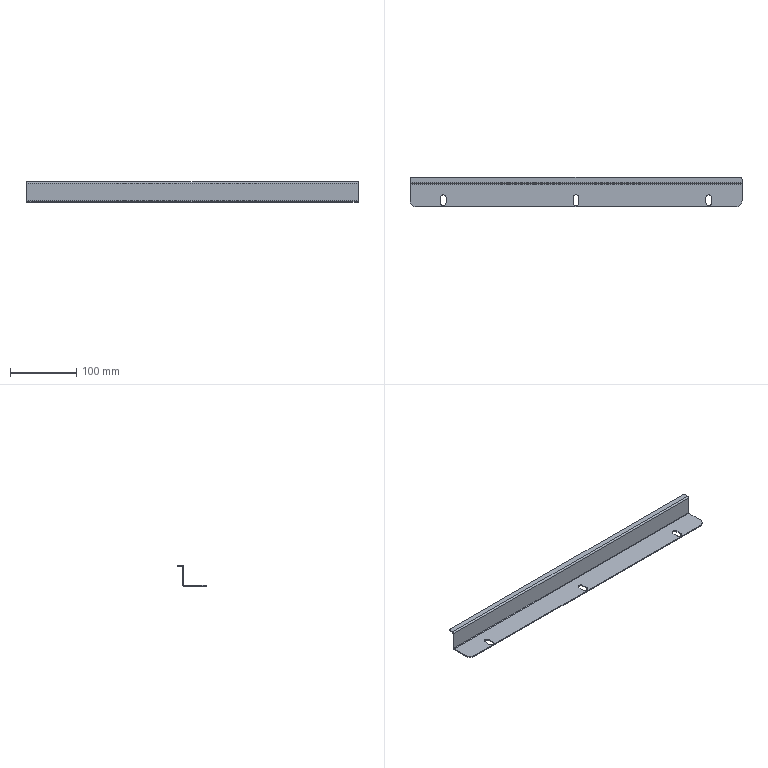Part | SolidWorks | features BaseBody 1 | 1 solid | 38 faces | box 500 x 45 x 31.5 mm | volume 54661 mm3 | plane 24 | cylinder 14 | commonest cylinder face diameters 8.5 x6 1.473 x2 4.473 x2 6 x2 20 x2
STEP:
#1=CARTESIAN_POINT('',(250.,19.,27.763));
#2=VERTEX_POINT('',#1);
#3=CARTESIAN_POINT('',(250.,17.5,27.763));
#4=VERTEX_POINT('',#3);
#5=CARTESIAN_POINT('',(250.,19.,27.763));
#6=DIRECTION('',(0.,-1.,0.));
#7=VECTOR('',#6,1000.);
#8=LINE('',#5,#7);
#9=EDGE_CURVE('',#2,#4,#8,.T.);
#10=ORIENTED_EDGE('',*,*,#9,.T.);
#11=CARTESIAN_POINT('',(250.,17.5,0.7366));
#12=VERTEX_POINT('',#11);
#13=CARTESIAN_POINT('',(250.,17.5,0.));
#14=DIRECTION('',(0.,0.,-1.));
#15=VECTOR('',#14,1000.);
#16=LINE('',#13,#15);
#17=EDGE_CURVE('',#4,#12,#16,.T.);
#18=ORIENTED_EDGE('',*,*,#17,.T.);
#19=CARTESIAN_POINT('',(250.,19.,0.7366));
#20=VERTEX_POINT('',#19);
#21=CARTESIAN_POINT('',(250.,17.5,0.7366));
#22=DIRECTION('',(0.,1.,0.));
#23=VECTOR('',#22,1000.);
#24=LINE('',#21,#23);
#25=EDGE_CURVE('',#12,#20,#24,.T.);
#26=ORIENTED_EDGE('',*,*,#25,.T.);
#27=CARTESIAN_POINT('',(250.,19.,0.));
#28=DIRECTION('',(0.,0.,-1.));
#29=VECTOR('',#28,1000.);
#30=LINE('',#27,#29);
#31=EDGE_CURVE('',#2,#20,#30,.T.);
#32=ORIENTED_EDGE('',*,*,#31,.F.);
#33=EDGE_LOOP('',(#10,#18,#26,#32));
#34=FACE_OUTER_BOUND('',#33,.T.);
#35=CARTESIAN_POINT('',(250.,19.,0.));
#36=DIRECTION('',(-1.,0.,0.));
#37=DIRECTION('',(0.,0.,1.));
#38=AXIS2_PLACEMENT_3D('',#35,#36,#37);
#39=PLANE('',#38);
#40=ADVANCED_FACE('',(#34),#39,.F.);
#41=CARTESIAN_POINT('',(-250.,19.,27.763));
#42=VERTEX_POINT('',#41);
#43=CARTESIAN_POINT('',(-250.,17.5,27.763));
#44=VERTEX_POINT('',#43);
#45=CARTESIAN_POINT('',(-250.,19.,27.763));
#46=DIRECTION('',(0.,-1.,0.));
#47=VECTOR('',#46,1000.);
#48=LINE('',#45,#47);
#49=EDGE_CURVE('',#42,#44,#48,.T.);
#50=ORIENTED_EDGE('',*,*,#49,.F.);
#51=CARTESIAN_POINT('',(-250.,19.,0.7366));
#52=VERTEX_POINT('',#51);
#53=CARTESIAN_POINT('',(-250.,19.,28.5));
#54=DIRECTION('',(0.,0.,1.));
#55=VECTOR('',#54,1000.);
#56=LINE('',#53,#55);
#57=EDGE_CURVE('',#52,#42,#56,.T.);
#58=ORIENTED_EDGE('',*,*,#57,.F.);
#59=CARTESIAN_POINT('',(-250.,17.5,0.7366));
#60=VERTEX_POINT('',#59);
#61=CARTESIAN_POINT('',(-250.,17.5,0.7366));
#62=DIRECTION('',(0.,1.,0.));
#63=VECTOR('',#62,1000.);
#64=LINE('',#61,#63);
#65=EDGE_CURVE('',#60,#52,#64,.T.);
#66=ORIENTED_EDGE('',*,*,#65,.F.);
#67=CARTESIAN_POINT('',(-250.,17.5,28.5));
#68=DIRECTION('',(0.,0.,1.));
#69=VECTOR('',#68,1000.);
#70=LINE('',#67,#69);
#71=EDGE_CURVE('',#60,#44,#70,.T.);
#72=ORIENTED_EDGE('',*,*,#71,.T.);
#73=EDGE_LOOP('',(#50,#58,#66,#72));
#74=FACE_OUTER_BOUND('',#73,.T.);
#75=CARTESIAN_POINT('',(-250.,19.,28.5));
#76=DIRECTION('',(1.,0.,0.));
#77=DIRECTION('',(0.,0.,-1.));
#78=AXIS2_PLACEMENT_3D('',#75,#76,#77);
#79=PLANE('',#78);
#80=ADVANCED_FACE('',(#74),#79,.F.);
#81=CARTESIAN_POINT('',(250.,19.,27.763));
#82=DIRECTION('',(-1.,0.,0.));
#83=VECTOR('',#82,1000.);
#84=LINE('',#81,#83);
#85=EDGE_CURVE('',#2,#42,#84,.T.);
#86=ORIENTED_EDGE('',*,*,#85,.F.);
#87=ORIENTED_EDGE('',*,*,#31,.T.);
#88=CARTESIAN_POINT('',(250.,19.,0.7366));
#89=DIRECTION('',(1.,0.,0.));
#90=VECTOR('',#89,1000.);
#91=LINE('',#88,#90);
#92=EDGE_CURVE('',#52,#20,#91,.T.);
#93=ORIENTED_EDGE('',*,*,#92,.F.);
#94=ORIENTED_EDGE('',*,*,#57,.T.);
#95=EDGE_LOOP('',(#86,#87,#93,#94));
#96=FACE_OUTER_BOUND('',#95,.T.);
#97=CARTESIAN_POINT('',(250.,19.,28.5));
#98=DIRECTION('',(0.,-1.,0.));
#99=DIRECTION('',(0.,0.,-1.));
#100=AXIS2_PLACEMENT_3D('',#97,#98,#99);
#101=PLANE('',#100);
#102=ADVANCED_FACE('',(#96),#101,.F.);
#103=ORIENTED_EDGE('',*,*,#17,.F.);
#104=CARTESIAN_POINT('',(250.,17.5,27.763));
#105=DIRECTION('',(-1.,0.,0.));
#106=VECTOR('',#105,1000.);
#107=LINE('',#104,#106);
#108=EDGE_CURVE('',#4,#44,#107,.T.);
#109=ORIENTED_EDGE('',*,*,#108,.T.);
#110=ORIENTED_EDGE('',*,*,#71,.F.);
#111=CARTESIAN_POINT('',(250.,17.5,0.7366));
#112=DIRECTION('',(-1.,0.,0.));
#113=VECTOR('',#112,1000.);
#114=LINE('',#111,#113);
#115=EDGE_CURVE('',#12,#60,#114,.T.);
#116=ORIENTED_EDGE('',*,*,#115,.F.);
#117=EDGE_LOOP('',(#103,#109,#110,#116));
#118=FACE_OUTER_BOUND('',#117,.T.);
#119=CARTESIAN_POINT('',(250.,17.5,28.5));
#120=DIRECTION('',(0.,-1.,0.));
#121=DIRECTION('',(0.,0.,-1.));
#122=AXIS2_PLACEMENT_3D('',#119,#120,#121);
#123=PLANE('',#122);
#124=ADVANCED_FACE('',(#118),#123,.T.);
#125=CARTESIAN_POINT('',(-250.,16.763,-1.5));
#126=VERTEX_POINT('',#125);
#127=CARTESIAN_POINT('',(-250.,-7.5,-1.5));
#128=VERTEX_POINT('',#127);
#129=CARTESIAN_POINT('',(-250.,17.5,-1.5));
#130=DIRECTION('',(0.,-1.,0.));
#131=VECTOR('',#130,1000.);
#132=LINE('',#129,#131);
#133=EDGE_CURVE('',#126,#128,#132,.T.);
#134=ORIENTED_EDGE('',*,*,#133,.T.);
#135=CARTESIAN_POINT('',(-250.,-7.5,0.));
#136=VERTEX_POINT('',#135);
#137=CARTESIAN_POINT('',(-250.,-7.5,-1.5));
#138=DIRECTION('',(0.,0.,1.));
#139=VECTOR('',#138,1000.);
#140=LINE('',#137,#139);
#141=EDGE_CURVE('',#128,#136,#140,.T.);
#142=ORIENTED_EDGE('',*,*,#141,.T.);
#143=CARTESIAN_POINT('',(-250.,16.763,0.));
#144=VERTEX_POINT('',#143);
#145=CARTESIAN_POINT('',(-250.,17.5,0.));
#146=DIRECTION('',(0.,-1.,0.));
#147=VECTOR('',#146,1000.);
#148=LINE('',#145,#147);
#149=EDGE_CURVE('',#144,#136,#148,.T.);
#150=ORIENTED_EDGE('',*,*,#149,.F.);
#151=CARTESIAN_POINT('',(-250.,16.763,0.));
#152=DIRECTION('',(0.,0.,-1.));
#153=VECTOR('',#152,1000.);
#154=LINE('',#151,#153);
#155=EDGE_CURVE('',#144,#126,#154,.T.);
#156=ORIENTED_EDGE('',*,*,#155,.T.);
#157=EDGE_LOOP('',(#134,#142,#150,#156));
#158=FACE_OUTER_BOUND('',#157,.T.);
#159=CARTESIAN_POINT('',(-250.,17.5,-1.5));
#160=DIRECTION('',(-1.,0.,0.));
#161=DIRECTION('',(0.,0.,1.));
#162=AXIS2_PLACEMENT_3D('',#159,#160,#161);
#163=PLANE('',#162);
#164=ADVANCED_FACE('',(#158),#163,.T.);
#165=CARTESIAN_POINT('',(4.25,-11.5,-1.5));
#166=VERTEX_POINT('',#165);
#167=CARTESIAN_POINT('',(-4.25,-11.5,-1.5));
#168=VERTEX_POINT('',#167);
#169=CARTESIAN_POINT('',(0.,-11.5,-1.5));
#170=DIRECTION('',(0.,0.,-1.));
#171=DIRECTION('',(-1.,0.,0.));
#172=AXIS2_PLACEMENT_3D('',#169,#170,#171);
#173=CIRCLE('',#172,4.25);
#174=EDGE_CURVE('',#166,#168,#173,.T.);
#175=ORIENTED_EDGE('',*,*,#174,.F.);
#176=CARTESIAN_POINT('',(4.25,-3.5,-1.5));
#177=VERTEX_POINT('',#176);
#178=CARTESIAN_POINT('',(4.25,-17.5,-1.5));
#179=DIRECTION('',(0.,-1.,0.));
#180=VECTOR('',#179,1000.);
#181=LINE('',#178,#180);
#182=EDGE_CURVE('',#177,#166,#181,.T.);
#183=ORIENTED_EDGE('',*,*,#182,.F.);
#184=CARTESIAN_POINT('',(-4.25,-3.5,-1.5));
#185=VERTEX_POINT('',#184);
#186=CARTESIAN_POINT('',(0.,-3.5,-1.5));
#187=DIRECTION('',(0.,0.,-1.));
#188=DIRECTION('',(-1.,0.,0.));
#189=AXIS2_PLACEMENT_3D('',#186,#187,#188);
#190=CIRCLE('',#189,4.25);
#191=EDGE_CURVE('',#185,#177,#190,.T.);
#192=ORIENTED_EDGE('',*,*,#191,.F.);
#193=CARTESIAN_POINT('',(-4.25,-17.5,-1.5));
#194=DIRECTION('',(0.,1.,0.));
#195=VECTOR('',#194,1000.);
#196=LINE('',#193,#195);
#197=EDGE_CURVE('',#168,#185,#196,.T.);
#198=ORIENTED_EDGE('',*,*,#197,.F.);
#199=EDGE_LOOP('',(#175,#183,#192,#198));
#200=FACE_BOUND('',#199,.T.);
#201=CARTESIAN_POINT('',(195.75,-3.5,-1.5));
#202=VERTEX_POINT('',#201);
#203=CARTESIAN_POINT('',(204.25,-3.5,-1.5));
#204=VERTEX_POINT('',#203);
#205=CARTESIAN_POINT('',(200.,-3.5,-1.5));
#206=DIRECTION('',(0.,0.,-1.));
#207=DIRECTION('',(-1.,0.,0.));
#208=AXIS2_PLACEMENT_3D('',#205,#206,#207);
#209=CIRCLE('',#208,4.25);
#210=EDGE_CURVE('',#202,#204,#209,.T.);
#211=ORIENTED_EDGE('',*,*,#210,.F.);
#212=CARTESIAN_POINT('',(195.75,-11.5,-1.5));
#213=VERTEX_POINT('',#212);
#214=CARTESIAN_POINT('',(195.75,-17.5,-1.5));
#215=DIRECTION('',(0.,1.,0.));
#216=VECTOR('',#215,1000.);
#217=LINE('',#214,#216);
#218=EDGE_CURVE('',#213,#202,#217,.T.);
#219=ORIENTED_EDGE('',*,*,#218,.F.);
#220=CARTESIAN_POINT('',(204.25,-11.5,-1.5));
#221=VERTEX_POINT('',#220);
#222=CARTESIAN_POINT('',(200.,-11.5,-1.5));
#223=DIRECTION('',(0.,0.,-1.));
#224=DIRECTION('',(-1.,0.,0.));
#225=AXIS2_PLACEMENT_3D('',#222,#223,#224);
#226=CIRCLE('',#225,4.25);
#227=EDGE_CURVE('',#221,#213,#226,.T.);
#228=ORIENTED_EDGE('',*,*,#227,.F.);
#229=CARTESIAN_POINT('',(204.25,-17.5,-1.5));
#230=DIRECTION('',(0.,-1.,0.));
#231=VECTOR('',#230,1000.);
#232=LINE('',#229,#231);
#233=EDGE_CURVE('',#204,#221,#232,.T.);
#234=ORIENTED_EDGE('',*,*,#233,.F.);
#235=EDGE_LOOP('',(#211,#219,#228,#234));
#236=FACE_BOUND('',#235,.T.);
#237=CARTESIAN_POINT('',(-204.25,-3.5,-1.5));
#238=VERTEX_POINT('',#237);
#239=CARTESIAN_POINT('',(-195.75,-3.5,-1.5));
#240=VERTEX_POINT('',#239);
#241=CARTESIAN_POINT('',(-200.,-3.5,-1.5));
#242=DIRECTION('',(0.,0.,-1.));
#243=DIRECTION('',(-1.,0.,0.));
#244=AXIS2_PLACEMENT_3D('',#241,#242,#243);
#245=CIRCLE('',#244,4.25);
#246=EDGE_CURVE('',#238,#240,#245,.T.);
#247=ORIENTED_EDGE('',*,*,#246,.F.);
#248=CARTESIAN_POINT('',(-204.25,-11.5,-1.5));
#249=VERTEX_POINT('',#248);
#250=CARTESIAN_POINT('',(-204.25,-17.5,-1.5));
#251=DIRECTION('',(0.,1.,0.));
#252=VECTOR('',#251,1000.);
#253=LINE('',#250,#252);
#254=EDGE_CURVE('',#249,#238,#253,.T.);
#255=ORIENTED_EDGE('',*,*,#254,.F.);
#256=CARTESIAN_POINT('',(-195.75,-11.5,-1.5));
#257=VERTEX_POINT('',#256);
#258=CARTESIAN_POINT('',(-200.,-11.5,-1.5));
#259=DIRECTION('',(0.,0.,-1.));
#260=DIRECTION('',(-1.,0.,0.));
#261=AXIS2_PLACEMENT_3D('',#258,#259,#260);
#262=CIRCLE('',#261,4.25);
#263=EDGE_CURVE('',#257,#249,#262,.T.);
#264=ORIENTED_EDGE('',*,*,#263,.F.);
#265=CARTESIAN_POINT('',(-195.75,-17.5,-1.5));
#266=DIRECTION('',(0.,-1.,0.));
#267=VECTOR('',#266,1000.);
#268=LINE('',#265,#267);
#269=EDGE_CURVE('',#240,#257,#268,.T.);
#270=ORIENTED_EDGE('',*,*,#269,.F.);
#271=EDGE_LOOP('',(#247,#255,#264,#270));
#272=FACE_BOUND('',#271,.T.);
#273=CARTESIAN_POINT('',(250.,-7.5,-1.5));
#274=VERTEX_POINT('',#273);
#275=CARTESIAN_POINT('',(250.,16.763,-1.5));
#276=VERTEX_POINT('',#275);
#277=CARTESIAN_POINT('',(250.,17.5,-1.5));
#278=DIRECTION('',(0.,1.,0.));
#279=VECTOR('',#278,1000.);
#280=LINE('',#277,#279);
#281=EDGE_CURVE('',#274,#276,#280,.T.);
#282=ORIENTED_EDGE('',*,*,#281,.F.);
#283=CARTESIAN_POINT('',(240.,-17.5,-1.5));
#284=VERTEX_POINT('',#283);
#285=CARTESIAN_POINT('',(240.,-7.5,-1.5));
#286=DIRECTION('',(0.,0.,-1.));
#287=DIRECTION('',(-1.,0.,0.));
#288=AXIS2_PLACEMENT_3D('',#285,#286,#287);
#289=CIRCLE('',#288,10.);
#290=EDGE_CURVE('',#274,#284,#289,.T.);
#291=ORIENTED_EDGE('',*,*,#290,.T.);
#292=CARTESIAN_POINT('',(-240.,-17.5,-1.5));
#293=VERTEX_POINT('',#292);
#294=CARTESIAN_POINT('',(250.,-17.5,-1.5));
#295=DIRECTION('',(1.,0.,0.));
#296=VECTOR('',#295,1000.);
#297=LINE('',#294,#296);
#298=EDGE_CURVE('',#293,#284,#297,.T.);
#299=ORIENTED_EDGE('',*,*,#298,.F.);
#300=CARTESIAN_POINT('',(-240.,-7.5,-1.5));
#301=DIRECTION('',(0.,0.,-1.));
#302=DIRECTION('',(-1.,0.,0.));
#303=AXIS2_PLACEMENT_3D('',#300,#301,#302);
#304=CIRCLE('',#303,10.);
#305=EDGE_CURVE('',#293,#128,#304,.T.);
#306=ORIENTED_EDGE('',*,*,#305,.T.);
#307=ORIENTED_EDGE('',*,*,#133,.F.);
#308=CARTESIAN_POINT('',(-250.,16.763,-1.5));
#309=DIRECTION('',(1.,0.,0.));
#310=VECTOR('',#309,1000.);
#311=LINE('',#308,#310);
#312=EDGE_CURVE('',#126,#276,#311,.T.);
#313=ORIENTED_EDGE('',*,*,#312,.T.);
#314=EDGE_LOOP('',(#282,#291,#299,#306,#307,#313));
#315=FACE_OUTER_BOUND('',#314,.T.);
#316=CARTESIAN_POINT('',(-250.,-17.5,-1.5));
#317=DIRECTION('',(0.,0.,-1.));
#318=DIRECTION('',(-1.,0.,0.));
#319=AXIS2_PLACEMENT_3D('',#316,#317,#318);
#320=PLANE('',#319);
#321=ADVANCED_FACE('',(#200,#236,#272,#315),#320,.T.);
#322=CARTESIAN_POINT('',(4.25,-11.5,0.));
#323=VERTEX_POINT('',#322);
#324=CARTESIAN_POINT('',(4.25,-3.5,0.));
#325=VERTEX_POINT('',#324);
#326=CARTESIAN_POINT('',(4.25,-11.5,0.));
#327=DIRECTION('',(0.,1.,0.));
#328=VECTOR('',#327,1000.);
#329=LINE('',#326,#328);
#330=EDGE_CURVE('',#323,#325,#329,.T.);
#331=ORIENTED_EDGE('',*,*,#330,.F.);
#332=CARTESIAN_POINT('',(-4.25,-11.5,0.));
#333=VERTEX_POINT('',#332);
#334=CARTESIAN_POINT('',(0.,-11.5,0.));
#335=DIRECTION('',(0.,0.,1.));
#336=DIRECTION('',(1.,0.,0.));
#337=AXIS2_PLACEMENT_3D('',#334,#335,#336);
#338=CIRCLE('',#337,4.25);
#339=EDGE_CURVE('',#333,#323,#338,.T.);
#340=ORIENTED_EDGE('',*,*,#339,.F.);
#341=CARTESIAN_POINT('',(-4.25,-3.5,0.));
#342=VERTEX_POINT('',#341);
#343=CARTESIAN_POINT('',(-4.25,-11.5,0.));
#344=DIRECTION('',(0.,-1.,0.));
#345=VECTOR('',#344,1000.);
#346=LINE('',#343,#345);
#347=EDGE_CURVE('',#342,#333,#346,.T.);
#348=ORIENTED_EDGE('',*,*,#347,.F.);
#349=CARTESIAN_POINT('',(0.,-3.5,0.));
#350=DIRECTION('',(0.,0.,1.));
#351=DIRECTION('',(1.,0.,0.));
#352=AXIS2_PLACEMENT_3D('',#349,#350,#351);
#353=CIRCLE('',#352,4.25);
#354=EDGE_CURVE('',#325,#342,#353,.T.);
#355=ORIENTED_EDGE('',*,*,#354,.F.);
#356=EDGE_LOOP('',(#331,#340,#348,#355));
#357=FACE_BOUND('',#356,.T.);
#358=CARTESIAN_POINT('',(195.75,-3.5,0.));
#359=VERTEX_POINT('',#358);
#360=CARTESIAN_POINT('',(195.75,-11.5,0.));
#361=VERTEX_POINT('',#360);
#362=CARTESIAN_POINT('',(195.75,-3.5,0.));
#363=DIRECTION('',(0.,-1.,0.));
#364=VECTOR('',#363,1000.);
#365=LINE('',#362,#364);
#366=EDGE_CURVE('',#359,#361,#365,.T.);
#367=ORIENTED_EDGE('',*,*,#366,.F.);
#368=CARTESIAN_POINT('',(204.25,-3.5,0.));
#369=VERTEX_POINT('',#368);
#370=CARTESIAN_POINT('',(200.,-3.5,0.));
#371=DIRECTION('',(0.,0.,1.));
#372=DIRECTION('',(-1.,0.,0.));
#373=AXIS2_PLACEMENT_3D('',#370,#371,#372);
#374=CIRCLE('',#373,4.25);
#375=EDGE_CURVE('',#369,#359,#374,.T.);
#376=ORIENTED_EDGE('',*,*,#375,.F.);
#377=CARTESIAN_POINT('',(204.25,-11.5,0.));
#378=VERTEX_POINT('',#377);
#379=CARTESIAN_POINT('',(204.25,-3.5,0.));
#380=DIRECTION('',(0.,1.,0.));
#381=VECTOR('',#380,1000.);
#382=LINE('',#379,#381);
#383=EDGE_CURVE('',#378,#369,#382,.T.);
#384=ORIENTED_EDGE('',*,*,#383,.F.);
#385=CARTESIAN_POINT('',(200.,-11.5,0.));
#386=DIRECTION('',(0.,0.,1.));
#387=DIRECTION('',(-1.,0.,0.));
#388=AXIS2_PLACEMENT_3D('',#385,#386,#387);
#389=CIRCLE('',#388,4.25);
#390=EDGE_CURVE('',#361,#378,#389,.T.);
#391=ORIENTED_EDGE('',*,*,#390,.F.);
#392=EDGE_LOOP('',(#367,#376,#384,#391));
#393=FACE_BOUND('',#392,.T.);
#394=CARTESIAN_POINT('',(-204.25,-3.5,0.));
#395=VERTEX_POINT('',#394);
#396=CARTESIAN_POINT('',(-204.25,-11.5,0.));
#397=VERTEX_POINT('',#396);
#398=CARTESIAN_POINT('',(-204.25,-3.5,0.));
#399=DIRECTION('',(0.,-1.,0.));
#400=VECTOR('',#399,1000.);
#401=LINE('',#398,#400);
#402=EDGE_CURVE('',#395,#397,#401,.T.);
#403=ORIENTED_EDGE('',*,*,#402,.F.);
#404=CARTESIAN_POINT('',(-195.75,-3.5,0.));
#405=VERTEX_POINT('',#404);
#406=CARTESIAN_POINT('',(-200.,-3.5,0.));
#407=DIRECTION('',(0.,0.,1.));
#408=DIRECTION('',(1.,0.,0.));
#409=AXIS2_PLACEMENT_3D('',#406,#407,#408);
#410=CIRCLE('',#409,4.25);
#411=EDGE_CURVE('',#405,#395,#410,.T.);
#412=ORIENTED_EDGE('',*,*,#411,.F.);
#413=CARTESIAN_POINT('',(-195.75,-11.5,0.));
#414=VERTEX_POINT('',#413);
#415=CARTESIAN_POINT('',(-195.75,-3.5,0.));
#416=DIRECTION('',(0.,1.,0.));
#417=VECTOR('',#416,1000.);
#418=LINE('',#415,#417);
#419=EDGE_CURVE('',#414,#405,#418,.T.);
#420=ORIENTED_EDGE('',*,*,#419,.F.);
#421=CARTESIAN_POINT('',(-200.,-11.5,0.));
#422=DIRECTION('',(0.,0.,1.));
#423=DIRECTION('',(1.,0.,0.));
#424=AXIS2_PLACEMENT_3D('',#421,#422,#423);
#425=CIRCLE('',#424,4.25);
#426=EDGE_CURVE('',#397,#414,#425,.T.);
#427=ORIENTED_EDGE('',*,*,#426,.F.);
#428=EDGE_LOOP('',(#403,#412,#420,#427));
#429=FACE_BOUND('',#428,.T.);
#430=CARTESIAN_POINT('',(-240.,-17.5,0.));
#431=VERTEX_POINT('',#430);
#432=CARTESIAN_POINT('',(240.,-17.5,0.));
#433=VERTEX_POINT('',#432);
#434=CARTESIAN_POINT('',(250.,-17.5,0.));
#435=DIRECTION('',(1.,0.,0.));
#436=VECTOR('',#435,1000.);
#437=LINE('',#434,#436);
#438=EDGE_CURVE('',#431,#433,#437,.T.);
#439=ORIENTED_EDGE('',*,*,#438,.T.);
#440=CARTESIAN_POINT('',(250.,-7.5,0.));
#441=VERTEX_POINT('',#440);
#442=CARTESIAN_POINT('',(240.,-7.5,0.));
#443=DIRECTION('',(0.,0.,1.));
#444=DIRECTION('',(-1.,0.,0.));
#445=AXIS2_PLACEMENT_3D('',#442,#443,#444);
#446=CIRCLE('',#445,10.);
#447=EDGE_CURVE('',#433,#441,#446,.T.);
#448=ORIENTED_EDGE('',*,*,#447,.T.);
#449=CARTESIAN_POINT('',(250.,16.763,0.));
#450=VERTEX_POINT('',#449);
#451=CARTESIAN_POINT('',(250.,17.5,0.));
#452=DIRECTION('',(0.,1.,0.));
#453=VECTOR('',#452,1000.);
#454=LINE('',#451,#453);
#455=EDGE_CURVE('',#441,#450,#454,.T.);
#456=ORIENTED_EDGE('',*,*,#455,.T.);
#457=CARTESIAN_POINT('',(-250.,16.763,0.));
#458=DIRECTION('',(1.,0.,0.));
#459=VECTOR('',#458,1000.);
#460=LINE('',#457,#459);
#461=EDGE_CURVE('',#144,#450,#460,.T.);
#462=ORIENTED_EDGE('',*,*,#461,.F.);
#463=ORIENTED_EDGE('',*,*,#149,.T.);
#464=CARTESIAN_POINT('',(-240.,-7.5,0.));
#465=DIRECTION('',(0.,0.,1.));
#466=DIRECTION('',(-1.,0.,0.));
#467=AXIS2_PLACEMENT_3D('',#464,#465,#466);
#468=CIRCLE('',#467,10.);
#469=EDGE_CURVE('',#136,#431,#468,.T.);
#470=ORIENTED_EDGE('',*,*,#469,.T.);
#471=EDGE_LOOP('',(#439,#448,#456,#462,#463,#470));
#472=FACE_OUTER_BOUND('',#471,.T.);
#473=CARTESIAN_POINT('',(-250.,-17.5,0.));
#474=DIRECTION('',(0.,0.,-1.));
#475=DIRECTION('',(-1.,0.,0.));
#476=AXIS2_PLACEMENT_3D('',#473,#474,#475);
#477=PLANE('',#476);
#478=ADVANCED_FACE('',(#357,#393,#429,#472),#477,.F.);
#479=ORIENTED_EDGE('',*,*,#455,.F.);
#480=CARTESIAN_POINT('',(250.,-7.5,-1.5));
#481=DIRECTION('',(0.,0.,-1.));
#482=VECTOR('',#481,1000.);
#483=LINE('',#480,#482);
#484=EDGE_CURVE('',#441,#274,#483,.T.);
#485=ORIENTED_EDGE('',*,*,#484,.T.);
#486=ORIENTED_EDGE('',*,*,#281,.T.);
#487=CARTESIAN_POINT('',(250.,16.763,0.));
#488=DIRECTION('',(0.,0.,-1.));
#489=VECTOR('',#488,1000.);
#490=LINE('',#487,#489);
#491=EDGE_CURVE('',#450,#276,#490,.T.);
#492=ORIENTED_EDGE('',*,*,#491,.F.);
#493=EDGE_LOOP('',(#479,#485,#486,#492));
#494=FACE_OUTER_BOUND('',#493,.T.);
#495=CARTESIAN_POINT('',(250.,17.5,-1.5));
#496=DIRECTION('',(1.,0.,0.));
#497=DIRECTION('',(0.,1.,0.));
#498=AXIS2_PLACEMENT_3D('',#495,#496,#497);
#499=PLANE('',#498);
#500=ADVANCED_FACE('',(#494),#499,.T.);
#501=ORIENTED_EDGE('',*,*,#298,.T.);
#502=CARTESIAN_POINT('',(240.,-17.5,-1.5));
#503=DIRECTION('',(0.,0.,1.));
#504=VECTOR('',#503,1000.);
#505=LINE('',#502,#504);
#506=EDGE_CURVE('',#284,#433,#505,.T.);
#507=ORIENTED_EDGE('',*,*,#506,.T.);
#508=ORIENTED_EDGE('',*,*,#438,.F.);
#509=CARTESIAN_POINT('',(-240.,-17.5,-1.5));
#510=DIRECTION('',(0.,0.,-1.));
#511=VECTOR('',#510,1000.);
#512=LINE('',#509,#511);
#513=EDGE_CURVE('',#431,#293,#512,.T.);
#514=ORIENTED_EDGE('',*,*,#513,.T.);
#515=EDGE_LOOP('',(#501,#507,#508,#514));
#516=FACE_OUTER_BOUND('',#515,.T.);
#517=CARTESIAN_POINT('',(250.,-17.5,-1.5));
#518=DIRECTION('',(0.,-1.,0.));
#519=DIRECTION('',(1.,0.,0.));
#520=AXIS2_PLACEMENT_3D('',#517,#518,#519);
#521=PLANE('',#520);
#522=ADVANCED_FACE('',(#516),#521,.T.);
#523=ORIENTED_EDGE('',*,*,#25,.F.);
#524=CARTESIAN_POINT('',(250.,16.763,0.7366));
#525=DIRECTION('',(1.,0.,0.));
#526=DIRECTION('',(0.,0.,1.));
#527=AXIS2_PLACEMENT_3D('',#524,#525,#526);
#528=CIRCLE('',#527,0.7366);
#529=EDGE_CURVE('',#450,#12,#528,.T.);
#530=ORIENTED_EDGE('',*,*,#529,.F.);
#531=ORIENTED_EDGE('',*,*,#491,.T.);
#532=CARTESIAN_POINT('',(250.,16.763,0.7366));
#533=DIRECTION('',(1.,0.,0.));
#534=DIRECTION('',(0.,0.,1.));
#535=AXIS2_PLACEMENT_3D('',#532,#533,#534);
#536=CIRCLE('',#535,2.237);
#537=EDGE_CURVE('',#276,#20,#536,.T.);
#538=ORIENTED_EDGE('',*,*,#537,.T.);
#539=EDGE_LOOP('',(#523,#530,#531,#538));
#540=FACE_OUTER_BOUND('',#539,.T.);
#541=CARTESIAN_POINT('',(250.,16.763,0.7366));
#542=DIRECTION('',(1.,0.,0.));
#543=DIRECTION('',(0.,0.,-1.));
#544=AXIS2_PLACEMENT_3D('',#541,#542,#543);
#545=PLANE('',#544);
#546=ADVANCED_FACE('',(#540),#545,.T.);
#547=CARTESIAN_POINT('',(-250.,16.763,0.7366));
#548=DIRECTION('',(-1.,0.,0.));
#549=DIRECTION('',(0.,0.,1.));
#550=AXIS2_PLACEMENT_3D('',#547,#548,#549);
#551=CIRCLE('',#550,0.7366);
#552=EDGE_CURVE('',#60,#144,#551,.T.);
#553=ORIENTED_EDGE('',*,*,#552,.F.);
#554=ORIENTED_EDGE('',*,*,#65,.T.);
#555=CARTESIAN_POINT('',(-250.,16.763,0.7366));
#556=DIRECTION('',(-1.,0.,0.));
#557=DIRECTION('',(0.,0.,1.));
#558=AXIS2_PLACEMENT_3D('',#555,#556,#557);
#559=CIRCLE('',#558,2.237);
#560=EDGE_CURVE('',#52,#126,#559,.T.);
#561=ORIENTED_EDGE('',*,*,#560,.T.);
#562=ORIENTED_EDGE('',*,*,#155,.F.);
#563=EDGE_LOOP('',(#553,#554,#561,#562));
#564=FACE_OUTER_BOUND('',#563,.T.);
#565=CARTESIAN_POINT('',(-250.,16.763,0.7366));
#566=DIRECTION('',(1.,0.,0.));
#567=DIRECTION('',(0.,0.,-1.));
#568=AXIS2_PLACEMENT_3D('',#565,#566,#567);
#569=PLANE('',#568);
#570=ADVANCED_FACE('',(#564),#569,.F.);
#571=ORIENTED_EDGE('',*,*,#312,.F.);
#572=ORIENTED_EDGE('',*,*,#560,.F.);
#573=ORIENTED_EDGE('',*,*,#92,.T.);
#574=ORIENTED_EDGE('',*,*,#537,.F.);
#575=EDGE_LOOP('',(#571,#572,#573,#574));
#576=FACE_OUTER_BOUND('',#575,.T.);
#577=CARTESIAN_POINT('',(-250.,16.763,0.7366));
#578=DIRECTION('',(-1.,0.,0.));
#579=DIRECTION('',(0.,1.,0.));
#580=AXIS2_PLACEMENT_3D('',#577,#578,#579);
#581=CYLINDRICAL_SURFACE('',#580,2.237);
#582=ADVANCED_FACE('',(#576),#581,.T.);
#583=ORIENTED_EDGE('',*,*,#461,.T.);
#584=ORIENTED_EDGE('',*,*,#529,.T.);
#585=ORIENTED_EDGE('',*,*,#115,.T.);
#586=ORIENTED_EDGE('',*,*,#552,.T.);
#587=EDGE_LOOP('',(#583,#584,#585,#586));
#588=FACE_OUTER_BOUND('',#587,.T.);
#589=CARTESIAN_POINT('',(-250.,16.763,0.7366));
#590=DIRECTION('',(-1.,0.,0.));
#591=DIRECTION('',(0.,1.,0.));
#592=AXIS2_PLACEMENT_3D('',#589,#590,#591);
#593=CYLINDRICAL_SURFACE('',#592,0.7366);
#594=ADVANCED_FACE('',(#588),#593,.F.);
#595=CARTESIAN_POINT('',(-250.,19.737,28.5));
#596=VERTEX_POINT('',#595);
#597=CARTESIAN_POINT('',(-250.,19.737,30.));
#598=VERTEX_POINT('',#597);
#599=CARTESIAN_POINT('',(-250.,19.737,28.5));
#600=DIRECTION('',(0.,0.,1.));
#601=VECTOR('',#600,1000.);
#602=LINE('',#599,#601);
#603=EDGE_CURVE('',#596,#598,#602,.T.);
#604=ORIENTED_EDGE('',*,*,#603,.F.);
#605=CARTESIAN_POINT('',(-250.,19.737,27.763));
#606=DIRECTION('',(-1.,0.,0.));
#607=DIRECTION('',(0.,0.,-1.));
#608=AXIS2_PLACEMENT_3D('',#605,#606,#607);
#609=CIRCLE('',#608,0.7366);
#610=EDGE_CURVE('',#42,#596,#609,.T.);
#611=ORIENTED_EDGE('',*,*,#610,.F.);
#612=ORIENTED_EDGE('',*,*,#49,.T.);
#613=CARTESIAN_POINT('',(-250.,19.737,27.763));
#614=DIRECTION('',(-1.,0.,0.));
#615=DIRECTION('',(0.,0.,-1.));
#616=AXIS2_PLACEMENT_3D('',#613,#614,#615);
#617=CIRCLE('',#616,2.237);
#618=EDGE_CURVE('',#44,#598,#617,.T.);
#619=ORIENTED_EDGE('',*,*,#618,.T.);
#620=EDGE_LOOP('',(#604,#611,#612,#619));
#621=FACE_OUTER_BOUND('',#620,.T.);
#622=CARTESIAN_POINT('',(-250.,19.737,27.763));
#623=DIRECTION('',(-1.,0.,0.));
#624=DIRECTION('',(0.,0.,1.));
#625=AXIS2_PLACEMENT_3D('',#622,#623,#624);
#626=PLANE('',#625);
#627=ADVANCED_FACE('',(#621),#626,.T.);
#628=CARTESIAN_POINT('',(250.,19.737,28.5));
#629=VERTEX_POINT('',#628);
#630=CARTESIAN_POINT('',(250.,19.737,27.763));
#631=DIRECTION('',(1.,0.,0.));
#632=DIRECTION('',(0.,0.,-1.));
#633=AXIS2_PLACEMENT_3D('',#630,#631,#632);
#634=CIRCLE('',#633,0.7366);
#635=EDGE_CURVE('',#629,#2,#634,.T.);
#636=ORIENTED_EDGE('',*,*,#635,.F.);
#637=CARTESIAN_POINT('',(250.,19.737,30.));
#638=VERTEX_POINT('',#637);
#639=CARTESIAN_POINT('',(250.,19.737,28.5));
#640=DIRECTION('',(0.,0.,1.));
#641=VECTOR('',#640,1000.);
#642=LINE('',#639,#641);
#643=EDGE_CURVE('',#629,#638,#642,.T.);
#644=ORIENTED_EDGE('',*,*,#643,.T.);
#645=CARTESIAN_POINT('',(250.,19.737,27.763));
#646=DIRECTION('',(1.,0.,0.));
#647=DIRECTION('',(0.,0.,-1.));
#648=AXIS2_PLACEMENT_3D('',#645,#646,#647);
#649=CIRCLE('',#648,2.237);
#650=EDGE_CURVE('',#638,#4,#649,.T.);
#651=ORIENTED_EDGE('',*,*,#650,.T.);
#652=ORIENTED_EDGE('',*,*,#9,.F.);
#653=EDGE_LOOP('',(#636,#644,#651,#652));
#654=FACE_OUTER_BOUND('',#653,.T.);
#655=CARTESIAN_POINT('',(250.,19.737,27.763));
#656=DIRECTION('',(-1.,0.,0.));
#657=DIRECTION('',(0.,0.,1.));
#658=AXIS2_PLACEMENT_3D('',#655,#656,#657);
#659=PLANE('',#658);
#660=ADVANCED_FACE('',(#654),#659,.F.);
#661=ORIENTED_EDGE('',*,*,#108,.F.);
#662=ORIENTED_EDGE('',*,*,#650,.F.);
#663=CARTESIAN_POINT('',(-250.,19.737,30.));
#664=DIRECTION('',(-1.,0.,0.));
#665=VECTOR('',#664,1000.);
#666=LINE('',#663,#665);
#667=EDGE_CURVE('',#638,#598,#666,.T.);
#668=ORIENTED_EDGE('',*,*,#667,.T.);
#669=ORIENTED_EDGE('',*,*,#618,.F.);
#670=EDGE_LOOP('',(#661,#662,#668,#669));
#671=FACE_OUTER_BOUND('',#670,.T.);
#672=CARTESIAN_POINT('',(250.,19.737,27.763));
#673=DIRECTION('',(1.,0.,0.));
#674=DIRECTION('',(0.,0.,1.));
#675=AXIS2_PLACEMENT_3D('',#672,#673,#674);
#676=CYLINDRICAL_SURFACE('',#675,2.237);
#677=ADVANCED_FACE('',(#671),#676,.T.);
#678=ORIENTED_EDGE('',*,*,#85,.T.);
#679=ORIENTED_EDGE('',*,*,#610,.T.);
#680=CARTESIAN_POINT('',(-250.,19.737,28.5));
#681=DIRECTION('',(1.,0.,0.));
#682=VECTOR('',#681,1000.);
#683=LINE('',#680,#682);
#684=EDGE_CURVE('',#596,#629,#683,.T.);
#685=ORIENTED_EDGE('',*,*,#684,.T.);
#686=ORIENTED_EDGE('',*,*,#635,.T.);
#687=EDGE_LOOP('',(#678,#679,#685,#686));
#688=FACE_OUTER_BOUND('',#687,.T.);
#689=CARTESIAN_POINT('',(250.,19.737,27.763));
#690=DIRECTION('',(1.,0.,0.));
#691=DIRECTION('',(0.,0.,1.));
#692=AXIS2_PLACEMENT_3D('',#689,#690,#691);
#693=CYLINDRICAL_SURFACE('',#692,0.7366);
#694=ADVANCED_FACE('',(#688),#693,.F.);
#695=CARTESIAN_POINT('',(-250.,24.5,30.));
#696=VERTEX_POINT('',#695);
#697=CARTESIAN_POINT('',(-250.,19.,30.));
#698=DIRECTION('',(0.,-1.,0.));
#699=VECTOR('',#698,1000.);
#700=LINE('',#697,#699);
#701=EDGE_CURVE('',#696,#598,#700,.T.);
#702=ORIENTED_EDGE('',*,*,#701,.F.);
#703=CARTESIAN_POINT('',(-250.,24.5,28.5));
#704=VERTEX_POINT('',#703);
#705=CARTESIAN_POINT('',(-250.,24.5,30.));
#706=DIRECTION('',(0.,0.,-1.));
#707=VECTOR('',#706,1000.);
#708=LINE('',#705,#707);
#709=EDGE_CURVE('',#696,#704,#708,.T.);
#710=ORIENTED_EDGE('',*,*,#709,.T.);
#711=CARTESIAN_POINT('',(-250.,19.,28.5));
#712=DIRECTION('',(0.,-1.,0.));
#713=VECTOR('',#712,1000.);
#714=LINE('',#711,#713);
#715=EDGE_CURVE('',#704,#596,#714,.T.);
#716=ORIENTED_EDGE('',*,*,#715,.T.);
#717=ORIENTED_EDGE('',*,*,#603,.T.);
#718=EDGE_LOOP('',(#702,#710,#716,#717));
#719=FACE_OUTER_BOUND('',#718,.T.);
#720=CARTESIAN_POINT('',(-250.,19.,30.));
#721=DIRECTION('',(1.,0.,0.));
#722=DIRECTION('',(0.,0.,-1.));
#723=AXIS2_PLACEMENT_3D('',#720,#721,#722);
#724=PLANE('',#723);
#725=ADVANCED_FACE('',(#719),#724,.F.);
#726=CARTESIAN_POINT('',(250.,24.5,28.5));
#727=VERTEX_POINT('',#726);
#728=CARTESIAN_POINT('',(250.,27.5,28.5));
#729=DIRECTION('',(0.,1.,0.));
#730=VECTOR('',#729,1000.);
#731=LINE('',#728,#730);
#732=EDGE_CURVE('',#629,#727,#731,.T.);
#733=ORIENTED_EDGE('',*,*,#732,.T.);
#734=CARTESIAN_POINT('',(250.,24.5,30.));
#735=VERTEX_POINT('',#734);
#736=CARTESIAN_POINT('',(250.,24.5,30.));
#737=DIRECTION('',(0.,0.,1.));
#738=VECTOR('',#737,1000.);
#739=LINE('',#736,#738);
#740=EDGE_CURVE('',#727,#735,#739,.T.);
#741=ORIENTED_EDGE('',*,*,#740,.T.);
#742=CARTESIAN_POINT('',(250.,27.5,30.));
#743=DIRECTION('',(0.,1.,0.));
#744=VECTOR('',#743,1000.);
#745=LINE('',#742,#744);
#746=EDGE_CURVE('',#638,#735,#745,.T.);
#747=ORIENTED_EDGE('',*,*,#746,.F.);
#748=ORIENTED_EDGE('',*,*,#643,.F.);
#749=EDGE_LOOP('',(#733,#741,#747,#748));
#750=FACE_OUTER_BOUND('',#749,.T.);
#751=CARTESIAN_POINT('',(250.,27.5,30.));
#752=DIRECTION('',(-1.,0.,0.));
#753=DIRECTION('',(0.,0.,1.));
#754=AXIS2_PLACEMENT_3D('',#751,#752,#753);
#755=PLANE('',#754);
#756=ADVANCED_FACE('',(#750),#755,.F.);
#757=ORIENTED_EDGE('',*,*,#746,.T.);
#758=CARTESIAN_POINT('',(247.,27.5,30.));
#759=VERTEX_POINT('',#758);
#760=CARTESIAN_POINT('',(247.,24.5,30.));
#761=DIRECTION('',(0.,0.,1.));
#762=DIRECTION('',(-1.,0.,0.));
#763=AXIS2_PLACEMENT_3D('',#760,#761,#762);
#764=CIRCLE('',#763,3.);
#765=EDGE_CURVE('',#735,#759,#764,.T.);
#766=ORIENTED_EDGE('',*,*,#765,.T.);
#767=CARTESIAN_POINT('',(-247.,27.5,30.));
#768=VERTEX_POINT('',#767);
#769=CARTESIAN_POINT('',(-250.,27.5,30.));
#770=DIRECTION('',(-1.,0.,0.));
#771=VECTOR('',#770,1000.);
#772=LINE('',#769,#771);
#773=EDGE_CURVE('',#759,#768,#772,.T.);
#774=ORIENTED_EDGE('',*,*,#773,.T.);
#775=CARTESIAN_POINT('',(-247.,24.5,30.));
#776=DIRECTION('',(0.,0.,1.));
#777=DIRECTION('',(-1.,0.,0.));
#778=AXIS2_PLACEMENT_3D('',#775,#776,#777);
#779=CIRCLE('',#778,3.);
#780=EDGE_CURVE('',#768,#696,#779,.T.);
#781=ORIENTED_EDGE('',*,*,#780,.T.);
#782=ORIENTED_EDGE('',*,*,#701,.T.);
#783=ORIENTED_EDGE('',*,*,#667,.F.);
#784=EDGE_LOOP('',(#757,#766,#774,#781,#782,#783));
#785=FACE_OUTER_BOUND('',#784,.T.);
#786=CARTESIAN_POINT('',(-250.,27.5,30.));
#787=DIRECTION('',(0.,0.,-1.));
#788=DIRECTION('',(-1.,0.,0.));
#789=AXIS2_PLACEMENT_3D('',#786,#787,#788);
#790=PLANE('',#789);
#791=ADVANCED_FACE('',(#785),#790,.F.);
#792=CARTESIAN_POINT('',(247.,27.5,28.5));
#793=VERTEX_POINT('',#792);
#794=CARTESIAN_POINT('',(-247.,27.5,28.5));
#795=VERTEX_POINT('',#794);
#796=CARTESIAN_POINT('',(-250.,27.5,28.5));
#797=DIRECTION('',(-1.,0.,0.));
#798=VECTOR('',#797,1000.);
#799=LINE('',#796,#798);
#800=EDGE_CURVE('',#793,#795,#799,.T.);
#801=ORIENTED_EDGE('',*,*,#800,.F.);
#802=CARTESIAN_POINT('',(247.,24.5,28.5));
#803=DIRECTION('',(0.,0.,-1.));
#804=DIRECTION('',(-1.,0.,0.));
#805=AXIS2_PLACEMENT_3D('',#802,#803,#804);
#806=CIRCLE('',#805,3.);
#807=EDGE_CURVE('',#793,#727,#806,.T.);
#808=ORIENTED_EDGE('',*,*,#807,.T.);
#809=ORIENTED_EDGE('',*,*,#732,.F.);
#810=ORIENTED_EDGE('',*,*,#684,.F.);
#811=ORIENTED_EDGE('',*,*,#715,.F.);
#812=CARTESIAN_POINT('',(-247.,24.5,28.5));
#813=DIRECTION('',(0.,0.,-1.));
#814=DIRECTION('',(-1.,0.,0.));
#815=AXIS2_PLACEMENT_3D('',#812,#813,#814);
#816=CIRCLE('',#815,3.);
#817=EDGE_CURVE('',#704,#795,#816,.T.);
#818=ORIENTED_EDGE('',*,*,#817,.T.);
#819=EDGE_LOOP('',(#801,#808,#809,#810,#811,#818));
#820=FACE_OUTER_BOUND('',#819,.T.);
#821=CARTESIAN_POINT('',(-250.,27.5,28.5));
#822=DIRECTION('',(0.,0.,-1.));
#823=DIRECTION('',(-1.,0.,0.));
#824=AXIS2_PLACEMENT_3D('',#821,#822,#823);
#825=PLANE('',#824);
#826=ADVANCED_FACE('',(#820),#825,.T.);
#827=ORIENTED_EDGE('',*,*,#773,.F.);
#828=CARTESIAN_POINT('',(247.,27.5,30.));
#829=DIRECTION('',(0.,0.,-1.));
#830=VECTOR('',#829,1000.);
#831=LINE('',#828,#830);
#832=EDGE_CURVE('',#759,#793,#831,.T.);
#833=ORIENTED_EDGE('',*,*,#832,.T.);
#834=ORIENTED_EDGE('',*,*,#800,.T.);
#835=CARTESIAN_POINT('',(-247.,27.5,30.));
#836=DIRECTION('',(0.,0.,1.));
#837=VECTOR('',#836,1000.);
#838=LINE('',#835,#837);
#839=EDGE_CURVE('',#795,#768,#838,.T.);
#840=ORIENTED_EDGE('',*,*,#839,.T.);
#841=EDGE_LOOP('',(#827,#833,#834,#840));
#842=FACE_OUTER_BOUND('',#841,.T.);
#843=CARTESIAN_POINT('',(-250.,27.5,30.));
#844=DIRECTION('',(0.,-1.,0.));
#845=DIRECTION('',(0.,0.,-1.));
#846=AXIS2_PLACEMENT_3D('',#843,#844,#845);
#847=PLANE('',#846);
#848=ADVANCED_FACE('',(#842),#847,.F.);
#849=ORIENTED_EDGE('',*,*,#246,.T.);
#850=CARTESIAN_POINT('',(-195.75,-3.5,-10.));
#851=DIRECTION('',(0.,0.,1.));
#852=VECTOR('',#851,1000.);
#853=LINE('',#850,#852);
#854=EDGE_CURVE('',#240,#405,#853,.T.);
#855=ORIENTED_EDGE('',*,*,#854,.T.);
#856=ORIENTED_EDGE('',*,*,#411,.T.);
#857=CARTESIAN_POINT('',(-204.25,-3.5,-10.));
#858=DIRECTION('',(0.,0.,1.));
#859=VECTOR('',#858,1000.);
#860=LINE('',#857,#859);
#861=EDGE_CURVE('',#238,#395,#860,.T.);
#862=ORIENTED_EDGE('',*,*,#861,.F.);
#863=EDGE_LOOP('',(#849,#855,#856,#862));
#864=FACE_OUTER_BOUND('',#863,.T.);
#865=CARTESIAN_POINT('',(-200.,-3.5,-10.));
#866=DIRECTION('',(0.,0.,1.));
#867=DIRECTION('',(1.,0.,0.));
#868=AXIS2_PLACEMENT_3D('',#865,#866,#867);
#869=CYLINDRICAL_SURFACE('',#868,4.25);
#870=ADVANCED_FACE('',(#864),#869,.F.);
#871=ORIENTED_EDGE('',*,*,#269,.T.);
#872=CARTESIAN_POINT('',(-195.75,-11.5,-10.));
#873=DIRECTION('',(0.,0.,1.));
#874=VECTOR('',#873,1000.);
#875=LINE('',#872,#874);
#876=EDGE_CURVE('',#257,#414,#875,.T.);
#877=ORIENTED_EDGE('',*,*,#876,.T.);
#878=ORIENTED_EDGE('',*,*,#419,.T.);
#879=ORIENTED_EDGE('',*,*,#854,.F.);
#880=EDGE_LOOP('',(#871,#877,#878,#879));
#881=FACE_OUTER_BOUND('',#880,.T.);
#882=CARTESIAN_POINT('',(-195.75,-3.5,-10.));
#883=DIRECTION('',(1.,0.,0.));
#884=DIRECTION('',(0.,0.,-1.));
#885=AXIS2_PLACEMENT_3D('',#882,#883,#884);
#886=PLANE('',#885);
#887=ADVANCED_FACE('',(#881),#886,.F.);
#888=ORIENTED_EDGE('',*,*,#263,.T.);
#889=CARTESIAN_POINT('',(-204.25,-11.5,-10.));
#890=DIRECTION('',(0.,0.,1.));
#891=VECTOR('',#890,1000.);
#892=LINE('',#889,#891);
#893=EDGE_CURVE('',#249,#397,#892,.T.);
#894=ORIENTED_EDGE('',*,*,#893,.T.);
#895=ORIENTED_EDGE('',*,*,#426,.T.);
#896=ORIENTED_EDGE('',*,*,#876,.F.);
#897=EDGE_LOOP('',(#888,#894,#895,#896));
#898=FACE_OUTER_BOUND('',#897,.T.);
#899=CARTESIAN_POINT('',(-200.,-11.5,-10.));
#900=DIRECTION('',(0.,0.,1.));
#901=DIRECTION('',(1.,0.,0.));
#902=AXIS2_PLACEMENT_3D('',#899,#900,#901);
#903=CYLINDRICAL_SURFACE('',#902,4.25);
#904=ADVANCED_FACE('',(#898),#903,.F.);
#905=ORIENTED_EDGE('',*,*,#254,.T.);
#906=ORIENTED_EDGE('',*,*,#861,.T.);
#907=ORIENTED_EDGE('',*,*,#402,.T.);
#908=ORIENTED_EDGE('',*,*,#893,.F.);
#909=EDGE_LOOP('',(#905,#906,#907,#908));
#910=FACE_OUTER_BOUND('',#909,.T.);
#911=CARTESIAN_POINT('',(-204.25,-3.5,-10.));
#912=DIRECTION('',(-1.,0.,0.));
#913=DIRECTION('',(0.,0.,1.));
#914=AXIS2_PLACEMENT_3D('',#911,#912,#913);
#915=PLANE('',#914);
#916=ADVANCED_FACE('',(#910),#915,.F.);
#917=ORIENTED_EDGE('',*,*,#210,.T.);
#918=CARTESIAN_POINT('',(204.25,-3.5,-10.));
#919=DIRECTION('',(0.,0.,1.));
#920=VECTOR('',#919,1000.);
#921=LINE('',#918,#920);
#922=EDGE_CURVE('',#204,#369,#921,.T.);
#923=ORIENTED_EDGE('',*,*,#922,.T.);
#924=ORIENTED_EDGE('',*,*,#375,.T.);
#925=CARTESIAN_POINT('',(195.75,-3.5,-10.));
#926=DIRECTION('',(0.,0.,1.));
#927=VECTOR('',#926,1000.);
#928=LINE('',#925,#927);
#929=EDGE_CURVE('',#202,#359,#928,.T.);
#930=ORIENTED_EDGE('',*,*,#929,.F.);
#931=EDGE_LOOP('',(#917,#923,#924,#930));
#932=FACE_OUTER_BOUND('',#931,.T.);
#933=CARTESIAN_POINT('',(200.,-3.5,-10.));
#934=DIRECTION('',(0.,0.,1.));
#935=DIRECTION('',(1.,0.,0.));
#936=AXIS2_PLACEMENT_3D('',#933,#934,#935);
#937=CYLINDRICAL_SURFACE('',#936,4.25);
#938=ADVANCED_FACE('',(#932),#937,.F.);
#939=ORIENTED_EDGE('',*,*,#233,.T.);
#940=CARTESIAN_POINT('',(204.25,-11.5,-10.));
#941=DIRECTION('',(0.,0.,1.));
#942=VECTOR('',#941,1000.);
#943=LINE('',#940,#942);
#944=EDGE_CURVE('',#221,#378,#943,.T.);
#945=ORIENTED_EDGE('',*,*,#944,.T.);
#946=ORIENTED_EDGE('',*,*,#383,.T.);
#947=ORIENTED_EDGE('',*,*,#922,.F.);
#948=EDGE_LOOP('',(#939,#945,#946,#947));
#949=FACE_OUTER_BOUND('',#948,.T.);
#950=CARTESIAN_POINT('',(204.25,-3.5,-10.));
#951=DIRECTION('',(1.,0.,0.));
#952=DIRECTION('',(0.,0.,-1.));
#953=AXIS2_PLACEMENT_3D('',#950,#951,#952);
#954=PLANE('',#953);
#955=ADVANCED_FACE('',(#949),#954,.F.);
#956=ORIENTED_EDGE('',*,*,#227,.T.);
#957=CARTESIAN_POINT('',(195.75,-11.5,-10.));
#958=DIRECTION('',(0.,0.,1.));
#959=VECTOR('',#958,1000.);
#960=LINE('',#957,#959);
#961=EDGE_CURVE('',#213,#361,#960,.T.);
#962=ORIENTED_EDGE('',*,*,#961,.T.);
#963=ORIENTED_EDGE('',*,*,#390,.T.);
#964=ORIENTED_EDGE('',*,*,#944,.F.);
#965=EDGE_LOOP('',(#956,#962,#963,#964));
#966=FACE_OUTER_BOUND('',#965,.T.);
#967=CARTESIAN_POINT('',(200.,-11.5,-10.));
#968=DIRECTION('',(0.,0.,1.));
#969=DIRECTION('',(1.,0.,0.));
#970=AXIS2_PLACEMENT_3D('',#967,#968,#969);
#971=CYLINDRICAL_SURFACE('',#970,4.25);
#972=ADVANCED_FACE('',(#966),#971,.F.);
#973=ORIENTED_EDGE('',*,*,#218,.T.);
#974=ORIENTED_EDGE('',*,*,#929,.T.);
#975=ORIENTED_EDGE('',*,*,#366,.T.);
#976=ORIENTED_EDGE('',*,*,#961,.F.);
#977=EDGE_LOOP('',(#973,#974,#975,#976));
#978=FACE_OUTER_BOUND('',#977,.T.);
#979=CARTESIAN_POINT('',(195.75,-3.5,-10.));
#980=DIRECTION('',(-1.,0.,0.));
#981=DIRECTION('',(0.,0.,1.));
#982=AXIS2_PLACEMENT_3D('',#979,#980,#981);
#983=PLANE('',#982);
#984=ADVANCED_FACE('',(#978),#983,.F.);
#985=ORIENTED_EDGE('',*,*,#174,.T.);
#986=CARTESIAN_POINT('',(-4.25,-11.5,-10.));
#987=DIRECTION('',(0.,0.,1.));
#988=VECTOR('',#987,1000.);
#989=LINE('',#986,#988);
#990=EDGE_CURVE('',#168,#333,#989,.T.);
#991=ORIENTED_EDGE('',*,*,#990,.T.);
#992=ORIENTED_EDGE('',*,*,#339,.T.);
#993=CARTESIAN_POINT('',(4.25,-11.5,-10.));
#994=DIRECTION('',(0.,0.,1.));
#995=VECTOR('',#994,1000.);
#996=LINE('',#993,#995);
#997=EDGE_CURVE('',#166,#323,#996,.T.);
#998=ORIENTED_EDGE('',*,*,#997,.F.);
#999=EDGE_LOOP('',(#985,#991,#992,#998));
#1000=FACE_OUTER_BOUND('',#999,.T.);
#1001=CARTESIAN_POINT('',(0.,-11.5,-10.));
#1002=DIRECTION('',(0.,0.,1.));
#1003=DIRECTION('',(1.,0.,0.));
#1004=AXIS2_PLACEMENT_3D('',#1001,#1002,#1003);
#1005=CYLINDRICAL_SURFACE('',#1004,4.25);
#1006=ADVANCED_FACE('',(#1000),#1005,.F.);
#1007=ORIENTED_EDGE('',*,*,#197,.T.);
#1008=CARTESIAN_POINT('',(-4.25,-3.5,-10.));
#1009=DIRECTION('',(0.,0.,1.));
#1010=VECTOR('',#1009,1000.);
#1011=LINE('',#1008,#1010);
#1012=EDGE_CURVE('',#185,#342,#1011,.T.);
#1013=ORIENTED_EDGE('',*,*,#1012,.T.);
#1014=ORIENTED_EDGE('',*,*,#347,.T.);
#1015=ORIENTED_EDGE('',*,*,#990,.F.);
#1016=EDGE_LOOP('',(#1007,#1013,#1014,#1015));
#1017=FACE_OUTER_BOUND('',#1016,.T.);
#1018=CARTESIAN_POINT('',(-4.25,-11.5,-10.));
#1019=DIRECTION('',(-1.,0.,0.));
#1020=DIRECTION('',(0.,-1.,0.));
#1021=AXIS2_PLACEMENT_3D('',#1018,#1019,#1020);
#1022=PLANE('',#1021);
#1023=ADVANCED_FACE('',(#1017),#1022,.F.);
#1024=ORIENTED_EDGE('',*,*,#191,.T.);
#1025=CARTESIAN_POINT('',(4.25,-3.5,-10.));
#1026=DIRECTION('',(0.,0.,1.));
#1027=VECTOR('',#1026,1000.);
#1028=LINE('',#1025,#1027);
#1029=EDGE_CURVE('',#177,#325,#1028,.T.);
#1030=ORIENTED_EDGE('',*,*,#1029,.T.);
#1031=ORIENTED_EDGE('',*,*,#354,.T.);
#1032=ORIENTED_EDGE('',*,*,#1012,.F.);
#1033=EDGE_LOOP('',(#1024,#1030,#1031,#1032));
#1034=FACE_OUTER_BOUND('',#1033,.T.);
#1035=CARTESIAN_POINT('',(0.,-3.5,-10.));
#1036=DIRECTION('',(0.,0.,1.));
#1037=DIRECTION('',(1.,0.,0.));
#1038=AXIS2_PLACEMENT_3D('',#1035,#1036,#1037);
#1039=CYLINDRICAL_SURFACE('',#1038,4.25);
#1040=ADVANCED_FACE('',(#1034),#1039,.F.);
#1041=ORIENTED_EDGE('',*,*,#182,.T.);
#1042=ORIENTED_EDGE('',*,*,#997,.T.);
#1043=ORIENTED_EDGE('',*,*,#330,.T.);
#1044=ORIENTED_EDGE('',*,*,#1029,.F.);
#1045=EDGE_LOOP('',(#1041,#1042,#1043,#1044));
#1046=FACE_OUTER_BOUND('',#1045,.T.);
#1047=CARTESIAN_POINT('',(4.25,-11.5,-10.));
#1048=DIRECTION('',(1.,0.,0.));
#1049=DIRECTION('',(0.,1.,0.));
#1050=AXIS2_PLACEMENT_3D('',#1047,#1048,#1049);
#1051=PLANE('',#1050);
#1052=ADVANCED_FACE('',(#1046),#1051,.F.);
#1053=ORIENTED_EDGE('',*,*,#290,.F.);
#1054=ORIENTED_EDGE('',*,*,#484,.F.);
#1055=ORIENTED_EDGE('',*,*,#447,.F.);
#1056=ORIENTED_EDGE('',*,*,#506,.F.);
#1057=EDGE_LOOP('',(#1053,#1054,#1055,#1056));
#1058=FACE_OUTER_BOUND('',#1057,.T.);
#1059=CARTESIAN_POINT('',(240.,-7.5,-1.5));
#1060=DIRECTION('',(0.,0.,1.));
#1061=DIRECTION('',(1.,0.,0.));
#1062=AXIS2_PLACEMENT_3D('',#1059,#1060,#1061);
#1063=CYLINDRICAL_SURFACE('',#1062,10.);
#1064=ADVANCED_FACE('',(#1058),#1063,.T.);
#1065=ORIENTED_EDGE('',*,*,#305,.F.);
#1066=ORIENTED_EDGE('',*,*,#513,.F.);
#1067=ORIENTED_EDGE('',*,*,#469,.F.);
#1068=ORIENTED_EDGE('',*,*,#141,.F.);
#1069=EDGE_LOOP('',(#1065,#1066,#1067,#1068));
#1070=FACE_OUTER_BOUND('',#1069,.T.);
#1071=CARTESIAN_POINT('',(-240.,-7.5,-1.5));
#1072=DIRECTION('',(0.,0.,1.));
#1073=DIRECTION('',(1.,0.,0.));
#1074=AXIS2_PLACEMENT_3D('',#1071,#1072,#1073);
#1075=CYLINDRICAL_SURFACE('',#1074,10.);
#1076=ADVANCED_FACE('',(#1070),#1075,.T.);
#1077=ORIENTED_EDGE('',*,*,#765,.F.);
#1078=ORIENTED_EDGE('',*,*,#740,.F.);
#1079=ORIENTED_EDGE('',*,*,#807,.F.);
#1080=ORIENTED_EDGE('',*,*,#832,.F.);
#1081=EDGE_LOOP('',(#1077,#1078,#1079,#1080));
#1082=FACE_OUTER_BOUND('',#1081,.T.);
#1083=CARTESIAN_POINT('',(247.,24.5,30.));
#1084=DIRECTION('',(0.,0.,-1.));
#1085=DIRECTION('',(-1.,0.,0.));
#1086=AXIS2_PLACEMENT_3D('',#1083,#1084,#1085);
#1087=CYLINDRICAL_SURFACE('',#1086,3.);
#1088=ADVANCED_FACE('',(#1082),#1087,.T.);
#1089=ORIENTED_EDGE('',*,*,#780,.F.);
#1090=ORIENTED_EDGE('',*,*,#839,.F.);
#1091=ORIENTED_EDGE('',*,*,#817,.F.);
#1092=ORIENTED_EDGE('',*,*,#709,.F.);
#1093=EDGE_LOOP('',(#1089,#1090,#1091,#1092));
#1094=FACE_OUTER_BOUND('',#1093,.T.);
#1095=CARTESIAN_POINT('',(-247.,24.5,30.));
#1096=DIRECTION('',(0.,0.,-1.));
#1097=DIRECTION('',(-1.,0.,0.));
#1098=AXIS2_PLACEMENT_3D('',#1095,#1096,#1097);
#1099=CYLINDRICAL_SURFACE('',#1098,3.);
#1100=ADVANCED_FACE('',(#1094),#1099,.T.);
#1101=CLOSED_SHELL('',(#40,#80,#102,#124,#164,#321,#478,#500,#522,#546,#570,#582,#594,#627,#660,#677,#694,#725,#756,#791,#826,#848,#870,#887,#904,#916,#938,#955,#972,#984,#1006,#1023,#1040,#1052,#1064,#1076,#1088,#1100));
#1102=MANIFOLD_SOLID_BREP('',#1101);
#1103=CARTESIAN_POINT('',(0.,0.,0.));
#1104=DIRECTION('',(0.,0.,1.));
#1105=DIRECTION('',(1.,0.,0.));
#1106=AXIS2_PLACEMENT_3D('',#1103,#1104,#1105);
#1107=(LENGTH_UNIT()NAMED_UNIT(*)SI_UNIT(.MILLI.,.METRE.));
#1108=UNCERTAINTY_MEASURE_WITH_UNIT(LENGTH_MEASURE(0.00001),#1107,'','');
#1109=(NAMED_UNIT(*)PLANE_ANGLE_UNIT()SI_UNIT($,.RADIAN.));
#1110=(NAMED_UNIT(*)SI_UNIT($,.STERADIAN.)SOLID_ANGLE_UNIT());
#1111=(GEOMETRIC_REPRESENTATION_CONTEXT(3)GLOBAL_UNCERTAINTY_ASSIGNED_CONTEXT((#1108))GLOBAL_UNIT_ASSIGNED_CONTEXT((#1107,#1109,#1110))REPRESENTATION_CONTEXT('',''));
#1112=ADVANCED_BREP_SHAPE_REPRESENTATION('',(#1102,#1106),#1111);